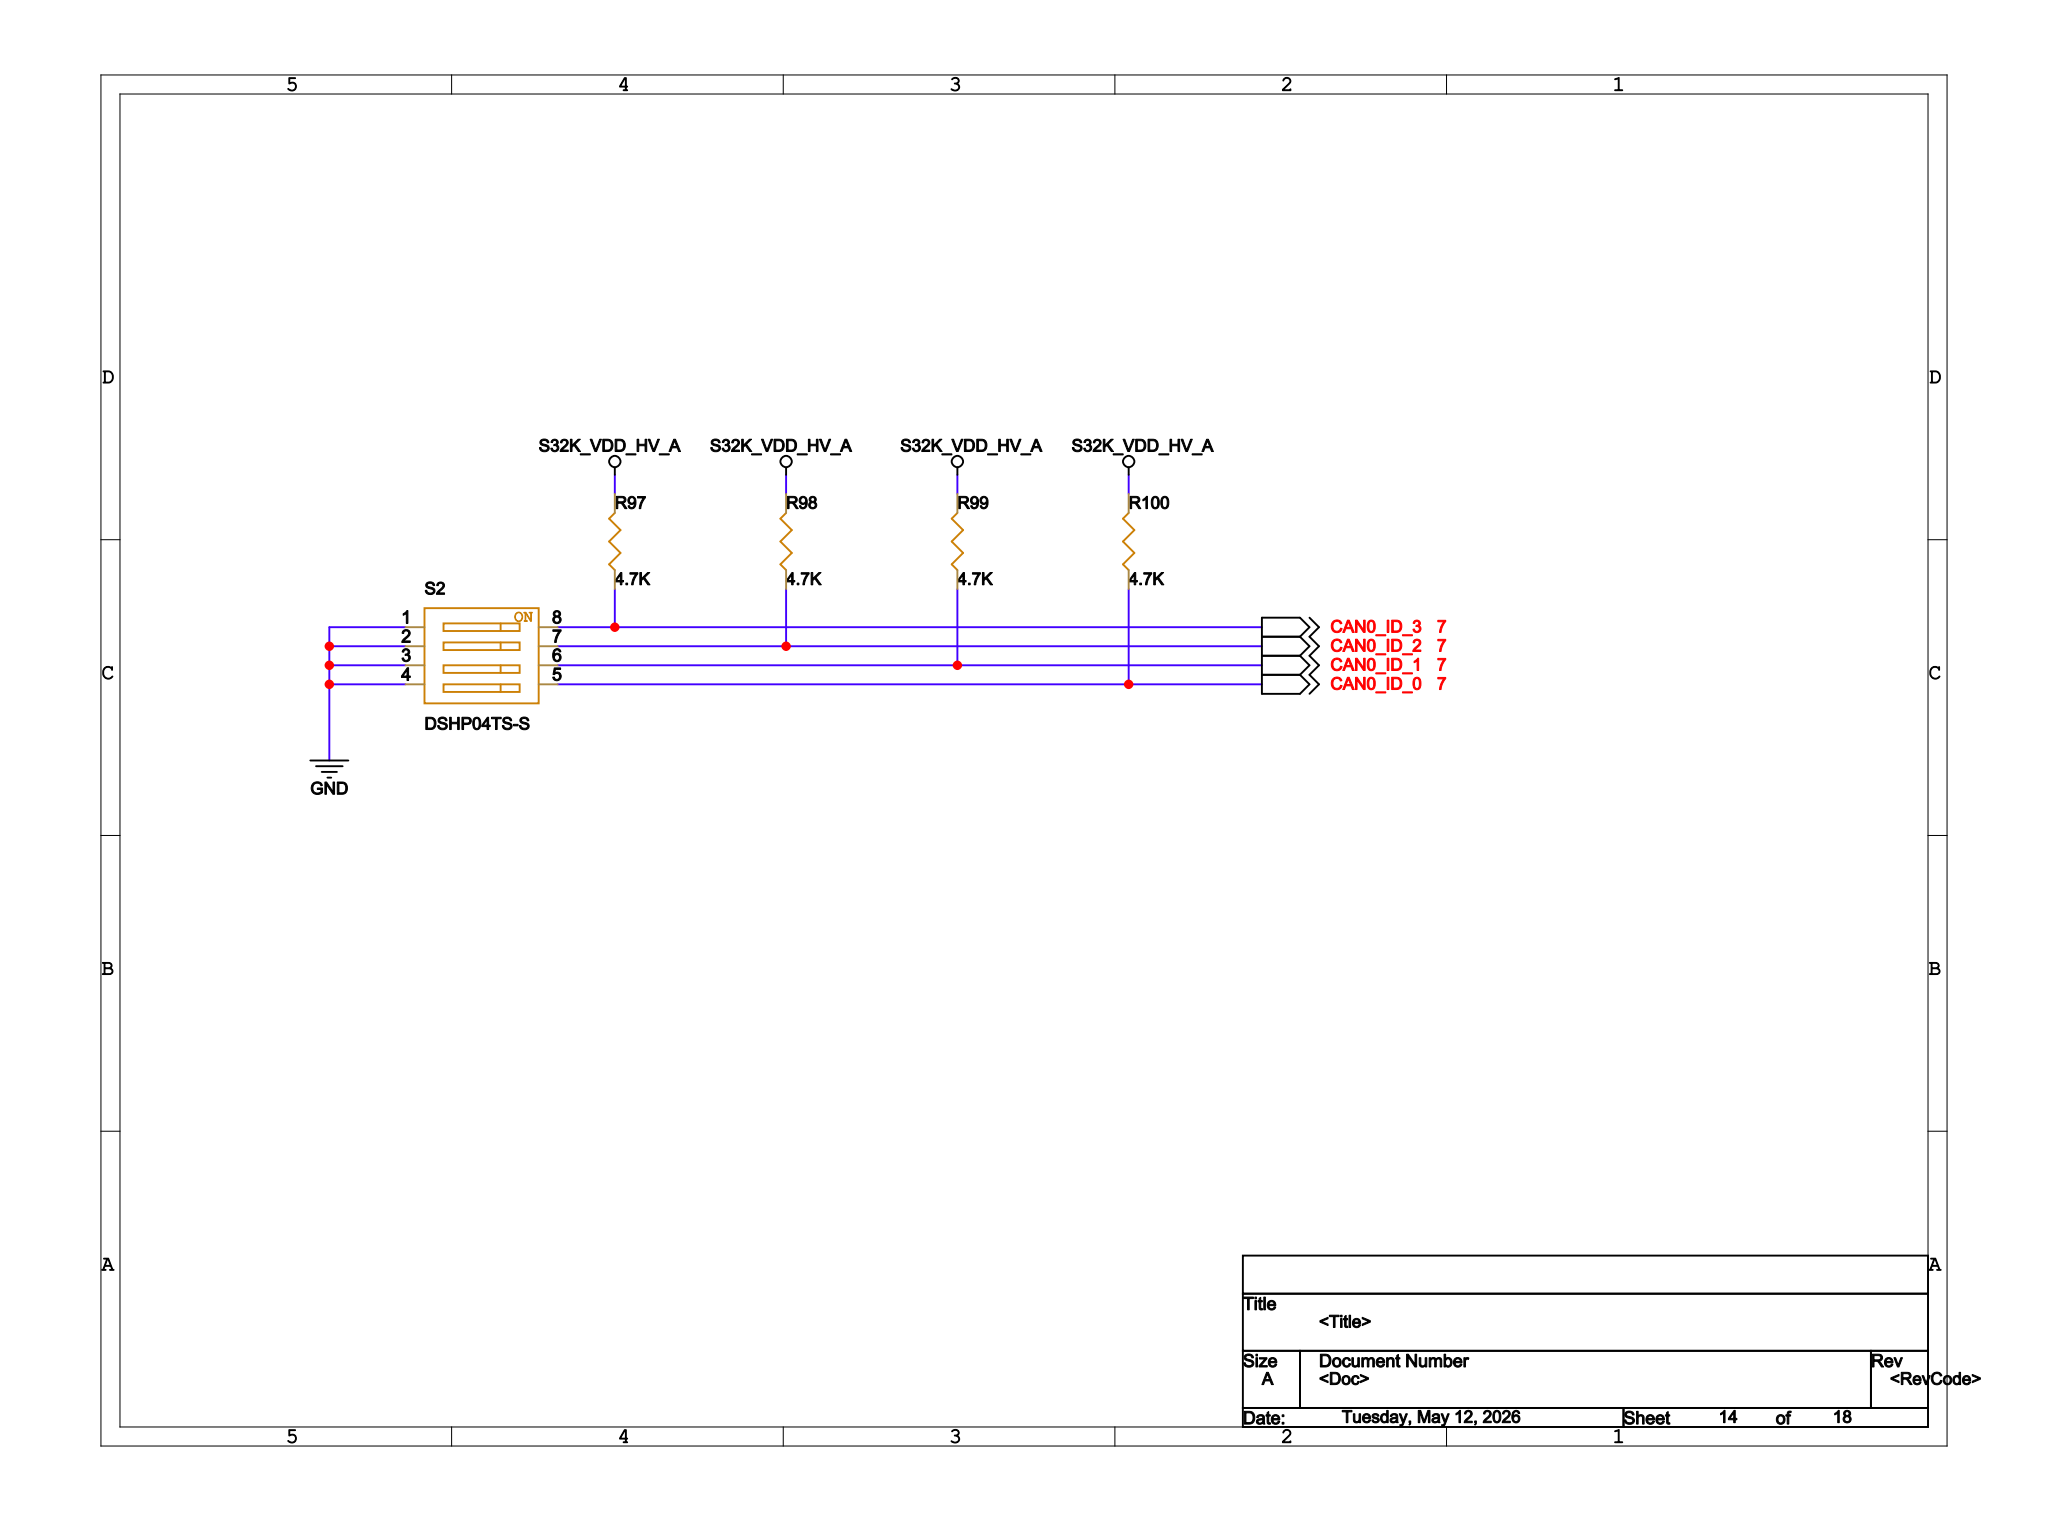Circuit board | Cadence Allegro | 330 parts | 215 nets | one sheet of the schematic
Parts on this sheet (reference | value | footprint):
R97 | 4.7K | 0402
R98 | 4.7K | 0402
R99 | 4.7K | 0402
R100 | 4.7K | 0402
S2 | DSHP04TS-S | DSHP04TS-S
Nets of these parts (net: part-pin ...):
GND: S2-1 S2-2 S2-3 S2-4
S32K_VDD_HV_A: R97-2 R98-2 R99-2 R100-2
CAN0_ID_0: R100-1 S2-5
CAN0_ID_3: R97-1 S2-8
CAN0_ID_2: R98-1 S2-7
CAN0_ID_1: R99-1 S2-6